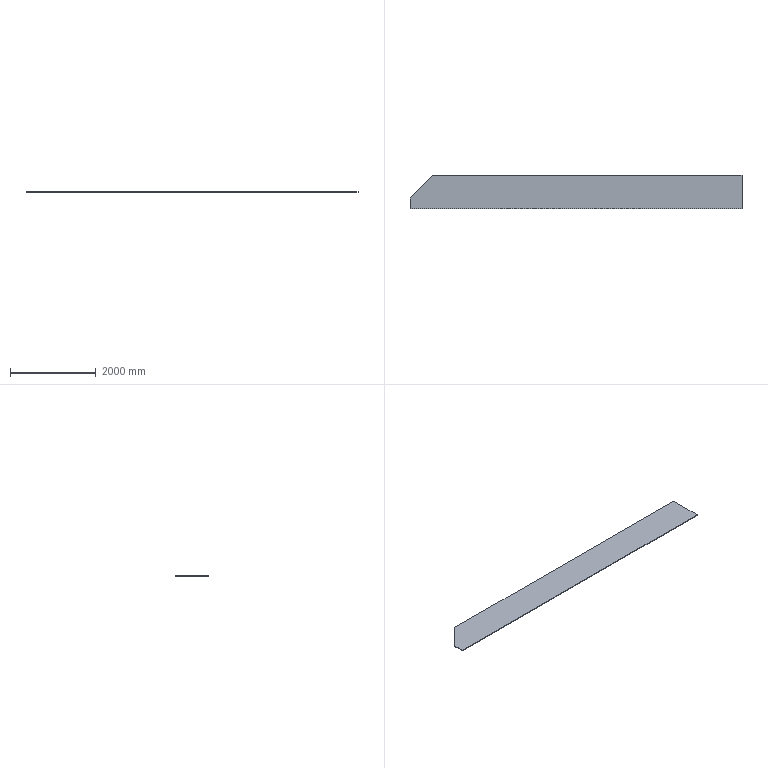Part | SolidWorks | features Extrusion 1 | 1 solid | 7 faces | box 7756 x 780 x 16 mm | volume 94547680 mm3 | plane 7
STEP:
#1=CARTESIAN_POINT('',(-7756.,0.,-8.));
#2=VERTEX_POINT('',#1);
#3=CARTESIAN_POINT('',(0.,0.,-8.));
#4=VERTEX_POINT('',#3);
#5=CARTESIAN_POINT('',(-7756.,0.,-8.));
#6=DIRECTION('',(1.,0.,0.));
#7=VECTOR('',#6,1000.);
#8=LINE('',#5,#7);
#9=EDGE_CURVE('',#2,#4,#8,.T.);
#10=ORIENTED_EDGE('',*,*,#9,.T.);
#11=CARTESIAN_POINT('',(0.,0.,8.));
#12=VERTEX_POINT('',#11);
#13=CARTESIAN_POINT('',(0.,0.,8.));
#14=DIRECTION('',(0.,0.,-1.));
#15=VECTOR('',#14,1000.);
#16=LINE('',#13,#15);
#17=EDGE_CURVE('',#12,#4,#16,.T.);
#18=ORIENTED_EDGE('',*,*,#17,.F.);
#19=CARTESIAN_POINT('',(-7756.,0.,8.));
#20=VERTEX_POINT('',#19);
#21=CARTESIAN_POINT('',(-7756.,0.,8.));
#22=DIRECTION('',(1.,0.,0.));
#23=VECTOR('',#22,1000.);
#24=LINE('',#21,#23);
#25=EDGE_CURVE('',#20,#12,#24,.T.);
#26=ORIENTED_EDGE('',*,*,#25,.F.);
#27=CARTESIAN_POINT('',(-7756.,0.,8.));
#28=DIRECTION('',(0.,0.,-1.));
#29=VECTOR('',#28,1000.);
#30=LINE('',#27,#29);
#31=EDGE_CURVE('',#20,#2,#30,.T.);
#32=ORIENTED_EDGE('',*,*,#31,.T.);
#33=EDGE_LOOP('',(#10,#18,#26,#32));
#34=FACE_OUTER_BOUND('',#33,.T.);
#35=CARTESIAN_POINT('',(-7756.,0.,8.));
#36=DIRECTION('',(0.,1.,0.));
#37=DIRECTION('',(0.,0.,1.));
#38=AXIS2_PLACEMENT_3D('',#35,#36,#37);
#39=PLANE('',#38);
#40=ADVANCED_FACE('',(#34),#39,.F.);
#41=CARTESIAN_POINT('',(0.,780.,-8.));
#42=VERTEX_POINT('',#41);
#43=CARTESIAN_POINT('',(0.,0.,-8.));
#44=DIRECTION('',(0.,1.,0.));
#45=VECTOR('',#44,1000.);
#46=LINE('',#43,#45);
#47=EDGE_CURVE('',#4,#42,#46,.T.);
#48=ORIENTED_EDGE('',*,*,#47,.T.);
#49=CARTESIAN_POINT('',(0.,780.,8.));
#50=VERTEX_POINT('',#49);
#51=CARTESIAN_POINT('',(0.,780.,8.));
#52=DIRECTION('',(0.,0.,-1.));
#53=VECTOR('',#52,1000.);
#54=LINE('',#51,#53);
#55=EDGE_CURVE('',#50,#42,#54,.T.);
#56=ORIENTED_EDGE('',*,*,#55,.F.);
#57=CARTESIAN_POINT('',(0.,0.,8.));
#58=DIRECTION('',(0.,1.,0.));
#59=VECTOR('',#58,1000.);
#60=LINE('',#57,#59);
#61=EDGE_CURVE('',#12,#50,#60,.T.);
#62=ORIENTED_EDGE('',*,*,#61,.F.);
#63=ORIENTED_EDGE('',*,*,#17,.T.);
#64=EDGE_LOOP('',(#48,#56,#62,#63));
#65=FACE_OUTER_BOUND('',#64,.T.);
#66=CARTESIAN_POINT('',(0.,0.,8.));
#67=DIRECTION('',(-1.,0.,0.));
#68=DIRECTION('',(0.,0.,1.));
#69=AXIS2_PLACEMENT_3D('',#66,#67,#68);
#70=PLANE('',#69);
#71=ADVANCED_FACE('',(#65),#70,.F.);
#72=CARTESIAN_POINT('',(-7226.,780.,-8.));
#73=VERTEX_POINT('',#72);
#74=CARTESIAN_POINT('',(0.,780.,-8.));
#75=DIRECTION('',(-1.,0.,0.));
#76=VECTOR('',#75,1000.);
#77=LINE('',#74,#76);
#78=EDGE_CURVE('',#42,#73,#77,.T.);
#79=ORIENTED_EDGE('',*,*,#78,.T.);
#80=CARTESIAN_POINT('',(-7226.,780.,8.));
#81=VERTEX_POINT('',#80);
#82=CARTESIAN_POINT('',(-7226.,780.,8.));
#83=DIRECTION('',(0.,0.,-1.));
#84=VECTOR('',#83,1000.);
#85=LINE('',#82,#84);
#86=EDGE_CURVE('',#81,#73,#85,.T.);
#87=ORIENTED_EDGE('',*,*,#86,.F.);
#88=CARTESIAN_POINT('',(0.,780.,8.));
#89=DIRECTION('',(-1.,0.,0.));
#90=VECTOR('',#89,1000.);
#91=LINE('',#88,#90);
#92=EDGE_CURVE('',#50,#81,#91,.T.);
#93=ORIENTED_EDGE('',*,*,#92,.F.);
#94=ORIENTED_EDGE('',*,*,#55,.T.);
#95=EDGE_LOOP('',(#79,#87,#93,#94));
#96=FACE_OUTER_BOUND('',#95,.T.);
#97=CARTESIAN_POINT('',(0.,780.,8.));
#98=DIRECTION('',(0.,-1.,0.));
#99=DIRECTION('',(1.,0.,0.));
#100=AXIS2_PLACEMENT_3D('',#97,#98,#99);
#101=PLANE('',#100);
#102=ADVANCED_FACE('',(#96),#101,.F.);
#103=CARTESIAN_POINT('',(-7756.,250.,-8.));
#104=VERTEX_POINT('',#103);
#105=CARTESIAN_POINT('',(-7226.,780.,-8.));
#106=DIRECTION('',(-0.7071,-0.7071,0.));
#107=VECTOR('',#106,1000.);
#108=LINE('',#105,#107);
#109=EDGE_CURVE('',#73,#104,#108,.T.);
#110=ORIENTED_EDGE('',*,*,#109,.T.);
#111=CARTESIAN_POINT('',(-7756.,250.,8.));
#112=VERTEX_POINT('',#111);
#113=CARTESIAN_POINT('',(-7756.,250.,8.));
#114=DIRECTION('',(0.,0.,-1.));
#115=VECTOR('',#114,1000.);
#116=LINE('',#113,#115);
#117=EDGE_CURVE('',#112,#104,#116,.T.);
#118=ORIENTED_EDGE('',*,*,#117,.F.);
#119=CARTESIAN_POINT('',(-7226.,780.,8.));
#120=DIRECTION('',(-0.7071,-0.7071,0.));
#121=VECTOR('',#120,1000.);
#122=LINE('',#119,#121);
#123=EDGE_CURVE('',#81,#112,#122,.T.);
#124=ORIENTED_EDGE('',*,*,#123,.F.);
#125=ORIENTED_EDGE('',*,*,#86,.T.);
#126=EDGE_LOOP('',(#110,#118,#124,#125));
#127=FACE_OUTER_BOUND('',#126,.T.);
#128=CARTESIAN_POINT('',(-7226.,780.,8.));
#129=DIRECTION('',(0.7071,-0.7071,0.));
#130=DIRECTION('',(0.7071,0.7071,0.));
#131=AXIS2_PLACEMENT_3D('',#128,#129,#130);
#132=PLANE('',#131);
#133=ADVANCED_FACE('',(#127),#132,.F.);
#134=CARTESIAN_POINT('',(-7756.,250.,-8.));
#135=DIRECTION('',(0.,-1.,0.));
#136=VECTOR('',#135,1000.);
#137=LINE('',#134,#136);
#138=EDGE_CURVE('',#104,#2,#137,.T.);
#139=ORIENTED_EDGE('',*,*,#138,.T.);
#140=ORIENTED_EDGE('',*,*,#31,.F.);
#141=CARTESIAN_POINT('',(-7756.,250.,8.));
#142=DIRECTION('',(0.,-1.,0.));
#143=VECTOR('',#142,1000.);
#144=LINE('',#141,#143);
#145=EDGE_CURVE('',#112,#20,#144,.T.);
#146=ORIENTED_EDGE('',*,*,#145,.F.);
#147=ORIENTED_EDGE('',*,*,#117,.T.);
#148=EDGE_LOOP('',(#139,#140,#146,#147));
#149=FACE_OUTER_BOUND('',#148,.T.);
#150=CARTESIAN_POINT('',(-7756.,250.,8.));
#151=DIRECTION('',(1.,0.,0.));
#152=DIRECTION('',(0.,0.,-1.));
#153=AXIS2_PLACEMENT_3D('',#150,#151,#152);
#154=PLANE('',#153);
#155=ADVANCED_FACE('',(#149),#154,.F.);
#156=ORIENTED_EDGE('',*,*,#25,.T.);
#157=ORIENTED_EDGE('',*,*,#61,.T.);
#158=ORIENTED_EDGE('',*,*,#92,.T.);
#159=ORIENTED_EDGE('',*,*,#123,.T.);
#160=ORIENTED_EDGE('',*,*,#145,.T.);
#161=EDGE_LOOP('',(#156,#157,#158,#159,#160));
#162=FACE_OUTER_BOUND('',#161,.T.);
#163=CARTESIAN_POINT('',(0.,0.,8.));
#164=DIRECTION('',(0.,0.,1.));
#165=DIRECTION('',(1.,0.,0.));
#166=AXIS2_PLACEMENT_3D('',#163,#164,#165);
#167=PLANE('',#166);
#168=ADVANCED_FACE('',(#162),#167,.T.);
#169=ORIENTED_EDGE('',*,*,#9,.F.);
#170=ORIENTED_EDGE('',*,*,#138,.F.);
#171=ORIENTED_EDGE('',*,*,#109,.F.);
#172=ORIENTED_EDGE('',*,*,#78,.F.);
#173=ORIENTED_EDGE('',*,*,#47,.F.);
#174=EDGE_LOOP('',(#169,#170,#171,#172,#173));
#175=FACE_OUTER_BOUND('',#174,.T.);
#176=CARTESIAN_POINT('',(0.,0.,-8.));
#177=DIRECTION('',(0.,0.,1.));
#178=DIRECTION('',(1.,0.,0.));
#179=AXIS2_PLACEMENT_3D('',#176,#177,#178);
#180=PLANE('',#179);
#181=ADVANCED_FACE('',(#175),#180,.F.);
#182=CLOSED_SHELL('',(#40,#71,#102,#133,#155,#168,#181));
#183=MANIFOLD_SOLID_BREP('',#182);
#184=CARTESIAN_POINT('',(0.,0.,0.));
#185=DIRECTION('',(0.,0.,1.));
#186=DIRECTION('',(1.,0.,0.));
#187=AXIS2_PLACEMENT_3D('',#184,#185,#186);
#188=(LENGTH_UNIT()NAMED_UNIT(*)SI_UNIT(.MILLI.,.METRE.));
#189=UNCERTAINTY_MEASURE_WITH_UNIT(LENGTH_MEASURE(0.00001),#188,'','');
#190=(NAMED_UNIT(*)PLANE_ANGLE_UNIT()SI_UNIT($,.RADIAN.));
#191=(NAMED_UNIT(*)SI_UNIT($,.STERADIAN.)SOLID_ANGLE_UNIT());
#192=(GEOMETRIC_REPRESENTATION_CONTEXT(3)GLOBAL_UNCERTAINTY_ASSIGNED_CONTEXT((#189))GLOBAL_UNIT_ASSIGNED_CONTEXT((#188,#190,#191))REPRESENTATION_CONTEXT('',''));
#193=ADVANCED_BREP_SHAPE_REPRESENTATION('',(#183,#187),#192);